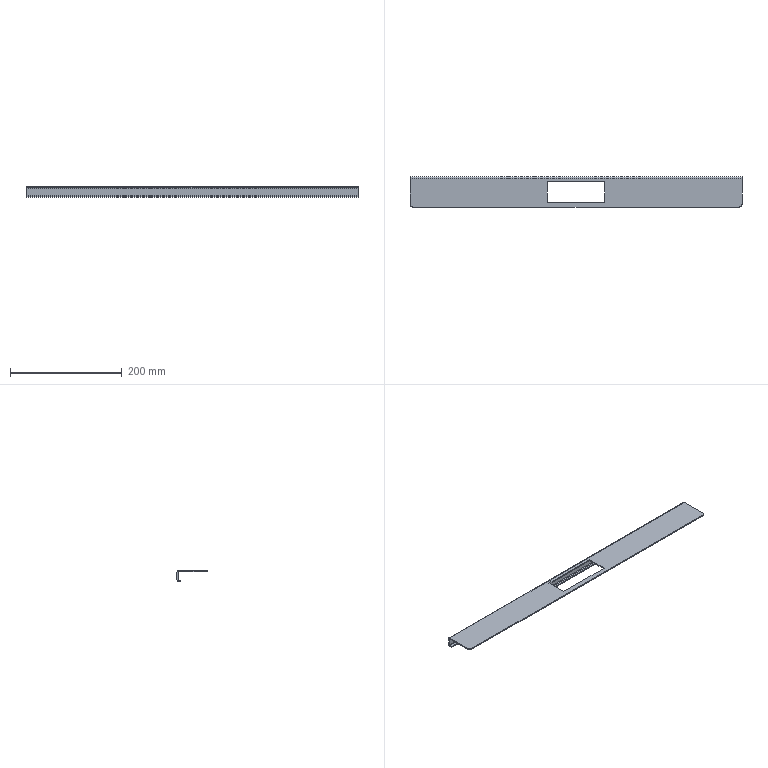Part | NX | 1 solid | 28 faces | box 595 x 54 x 19 mm | volume 80754 mm3 | plane 22 | cylinder 6 | commonest cylinder face diameters 2 x2 6 x2 10 x2
STEP:
#1=CARTESIAN_POINT('',(297.5,48.,87.));
#2=VERTEX_POINT('',#1);
#3=CARTESIAN_POINT('',(297.5,48.,100.));
#4=VERTEX_POINT('',#3);
#5=CARTESIAN_POINT('',(297.5,48.,101.));
#6=DIRECTION('',(0.,0.,1.));
#7=VECTOR('',#6,1000.);
#8=LINE('',#5,#7);
#9=EDGE_CURVE('',#2,#4,#8,.T.);
#10=ORIENTED_EDGE('',*,*,#9,.F.);
#11=CARTESIAN_POINT('',(297.5,50.,87.));
#12=VERTEX_POINT('',#11);
#13=CARTESIAN_POINT('',(297.5,48.,87.));
#14=DIRECTION('',(0.,1.,0.));
#15=VECTOR('',#14,1000.);
#16=LINE('',#13,#15);
#17=EDGE_CURVE('',#2,#12,#16,.T.);
#18=ORIENTED_EDGE('',*,*,#17,.T.);
#19=CARTESIAN_POINT('',(297.5,50.,100.));
#20=VERTEX_POINT('',#19);
#21=CARTESIAN_POINT('',(297.5,50.,101.));
#22=DIRECTION('',(0.,0.,1.));
#23=VECTOR('',#22,1000.);
#24=LINE('',#21,#23);
#25=EDGE_CURVE('',#12,#20,#24,.T.);
#26=ORIENTED_EDGE('',*,*,#25,.T.);
#27=CARTESIAN_POINT('',(297.5,48.,100.));
#28=DIRECTION('',(0.,1.,0.));
#29=VECTOR('',#28,1000.);
#30=LINE('',#27,#29);
#31=EDGE_CURVE('',#4,#20,#30,.T.);
#32=ORIENTED_EDGE('',*,*,#31,.F.);
#33=EDGE_LOOP('',(#10,#18,#26,#32));
#34=FACE_BOUND('',#33,.T.);
#35=CARTESIAN_POINT('',(297.5,50.,101.));
#36=DIRECTION('',(1.,0.,0.));
#37=DIRECTION('',(0.,0.,-1.));
#38=AXIS2_PLACEMENT_3D('',#35,#36,#37);
#39=PLANE('',#38);
#40=ADVANCED_FACE('',(#34),#39,.T.);
#41=ORIENTED_EDGE('',*,*,#25,.F.);
#42=CARTESIAN_POINT('',(-297.5,50.,87.));
#43=VERTEX_POINT('',#42);
#44=CARTESIAN_POINT('',(297.5,50.,87.));
#45=DIRECTION('',(1.,0.,0.));
#46=VECTOR('',#45,1000.);
#47=LINE('',#44,#46);
#48=EDGE_CURVE('',#12,#43,#47,.F.);
#49=ORIENTED_EDGE('',*,*,#48,.T.);
#50=CARTESIAN_POINT('',(-297.5,50.,100.));
#51=VERTEX_POINT('',#50);
#52=CARTESIAN_POINT('',(-297.5,50.,86.));
#53=DIRECTION('',(0.,0.,-1.));
#54=VECTOR('',#53,1000.);
#55=LINE('',#52,#54);
#56=EDGE_CURVE('',#51,#43,#55,.T.);
#57=ORIENTED_EDGE('',*,*,#56,.F.);
#58=CARTESIAN_POINT('',(0.,50.,100.));
#59=DIRECTION('',(1.,0.,0.));
#60=VECTOR('',#59,1000.);
#61=LINE('',#58,#60);
#62=EDGE_CURVE('',#51,#20,#61,.T.);
#63=ORIENTED_EDGE('',*,*,#62,.T.);
#64=EDGE_LOOP('',(#41,#49,#57,#63));
#65=FACE_BOUND('',#64,.T.);
#66=CARTESIAN_POINT('',(0.,50.,0.));
#67=DIRECTION('',(0.,1.,0.));
#68=DIRECTION('',(0.,0.,1.));
#69=AXIS2_PLACEMENT_3D('',#66,#67,#68);
#70=PLANE('',#69);
#71=ADVANCED_FACE('',(#65),#70,.T.);
#72=CARTESIAN_POINT('',(-297.5,48.,87.));
#73=VERTEX_POINT('',#72);
#74=CARTESIAN_POINT('',(297.5,48.,87.));
#75=DIRECTION('',(1.,0.,0.));
#76=VECTOR('',#75,1000.);
#77=LINE('',#74,#76);
#78=EDGE_CURVE('',#2,#73,#77,.F.);
#79=ORIENTED_EDGE('',*,*,#78,.F.);
#80=ORIENTED_EDGE('',*,*,#9,.T.);
#81=CARTESIAN_POINT('',(-297.5,48.,100.));
#82=VERTEX_POINT('',#81);
#83=CARTESIAN_POINT('',(-297.5,48.,100.));
#84=DIRECTION('',(1.,0.,0.));
#85=VECTOR('',#84,1000.);
#86=LINE('',#83,#85);
#87=EDGE_CURVE('',#82,#4,#86,.T.);
#88=ORIENTED_EDGE('',*,*,#87,.F.);
#89=CARTESIAN_POINT('',(-297.5,48.,86.));
#90=DIRECTION('',(0.,0.,-1.));
#91=VECTOR('',#90,1000.);
#92=LINE('',#89,#91);
#93=EDGE_CURVE('',#82,#73,#92,.T.);
#94=ORIENTED_EDGE('',*,*,#93,.T.);
#95=EDGE_LOOP('',(#79,#80,#88,#94));
#96=FACE_BOUND('',#95,.T.);
#97=CARTESIAN_POINT('',(0.,48.,0.));
#98=DIRECTION('',(0.,1.,0.));
#99=DIRECTION('',(0.,0.,1.));
#100=AXIS2_PLACEMENT_3D('',#97,#98,#99);
#101=PLANE('',#100);
#102=ADVANCED_FACE('',(#96),#101,.F.);
#103=CARTESIAN_POINT('',(297.5,1.,103.));
#104=VERTEX_POINT('',#103);
#105=CARTESIAN_POINT('',(297.5,47.,103.));
#106=VERTEX_POINT('',#105);
#107=CARTESIAN_POINT('',(297.5,48.,103.));
#108=DIRECTION('',(0.,1.,0.));
#109=VECTOR('',#108,1000.);
#110=LINE('',#107,#109);
#111=EDGE_CURVE('',#104,#106,#110,.T.);
#112=ORIENTED_EDGE('',*,*,#111,.F.);
#113=CARTESIAN_POINT('',(297.5,1.,101.));
#114=VERTEX_POINT('',#113);
#115=CARTESIAN_POINT('',(297.5,1.,103.));
#116=DIRECTION('',(0.,0.,-1.));
#117=VECTOR('',#116,1000.);
#118=LINE('',#115,#117);
#119=EDGE_CURVE('',#104,#114,#118,.T.);
#120=ORIENTED_EDGE('',*,*,#119,.T.);
#121=CARTESIAN_POINT('',(297.5,47.,101.));
#122=VERTEX_POINT('',#121);
#123=CARTESIAN_POINT('',(297.5,48.,101.));
#124=DIRECTION('',(0.,1.,0.));
#125=VECTOR('',#124,1000.);
#126=LINE('',#123,#125);
#127=EDGE_CURVE('',#114,#122,#126,.T.);
#128=ORIENTED_EDGE('',*,*,#127,.T.);
#129=CARTESIAN_POINT('',(297.5,47.,101.));
#130=DIRECTION('',(0.,0.,1.));
#131=VECTOR('',#130,1000.);
#132=LINE('',#129,#131);
#133=EDGE_CURVE('',#122,#106,#132,.T.);
#134=ORIENTED_EDGE('',*,*,#133,.T.);
#135=EDGE_LOOP('',(#112,#120,#128,#134));
#136=FACE_BOUND('',#135,.T.);
#137=CARTESIAN_POINT('',(297.5,48.,103.));
#138=DIRECTION('',(-1.,0.,0.));
#139=DIRECTION('',(0.,0.,1.));
#140=AXIS2_PLACEMENT_3D('',#137,#138,#139);
#141=PLANE('',#140);
#142=ADVANCED_FACE('',(#136),#141,.F.);
#143=CARTESIAN_POINT('',(-297.5,47.,101.));
#144=VERTEX_POINT('',#143);
#145=CARTESIAN_POINT('',(-297.5,1.,101.));
#146=VERTEX_POINT('',#145);
#147=CARTESIAN_POINT('',(-297.5,48.,101.));
#148=DIRECTION('',(0.,-1.,0.));
#149=VECTOR('',#148,1000.);
#150=LINE('',#147,#149);
#151=EDGE_CURVE('',#144,#146,#150,.T.);
#152=ORIENTED_EDGE('',*,*,#151,.T.);
#153=CARTESIAN_POINT('',(-297.5,1.,103.));
#154=VERTEX_POINT('',#153);
#155=CARTESIAN_POINT('',(-297.5,1.,103.));
#156=DIRECTION('',(0.,0.,-1.));
#157=VECTOR('',#156,1000.);
#158=LINE('',#155,#157);
#159=EDGE_CURVE('',#146,#154,#158,.F.);
#160=ORIENTED_EDGE('',*,*,#159,.T.);
#161=CARTESIAN_POINT('',(-297.5,47.,103.));
#162=VERTEX_POINT('',#161);
#163=CARTESIAN_POINT('',(-297.5,48.,103.));
#164=DIRECTION('',(0.,-1.,0.));
#165=VECTOR('',#164,1000.);
#166=LINE('',#163,#165);
#167=EDGE_CURVE('',#162,#154,#166,.T.);
#168=ORIENTED_EDGE('',*,*,#167,.F.);
#169=CARTESIAN_POINT('',(-297.5,47.,101.));
#170=DIRECTION('',(0.,0.,1.));
#171=VECTOR('',#170,1000.);
#172=LINE('',#169,#171);
#173=EDGE_CURVE('',#144,#162,#172,.T.);
#174=ORIENTED_EDGE('',*,*,#173,.F.);
#175=EDGE_LOOP('',(#152,#160,#168,#174));
#176=FACE_BOUND('',#175,.T.);
#177=CARTESIAN_POINT('',(-297.5,48.,103.));
#178=DIRECTION('',(1.,0.,0.));
#179=DIRECTION('',(0.,0.,-1.));
#180=AXIS2_PLACEMENT_3D('',#177,#178,#179);
#181=PLANE('',#180);
#182=ADVANCED_FACE('',(#176),#181,.F.);
#183=CARTESIAN_POINT('',(-51.5,41.5,103.));
#184=VERTEX_POINT('',#183);
#185=CARTESIAN_POINT('',(-51.5,4.5,103.));
#186=VERTEX_POINT('',#185);
#187=CARTESIAN_POINT('',(-51.5,4.5,103.));
#188=DIRECTION('',(0.,-1.,0.));
#189=VECTOR('',#188,1000.);
#190=LINE('',#187,#189);
#191=EDGE_CURVE('',#184,#186,#190,.T.);
#192=ORIENTED_EDGE('',*,*,#191,.F.);
#193=CARTESIAN_POINT('',(51.5,41.5,103.));
#194=VERTEX_POINT('',#193);
#195=CARTESIAN_POINT('',(51.5,41.5,103.));
#196=DIRECTION('',(-1.,0.,0.));
#197=VECTOR('',#196,1000.);
#198=LINE('',#195,#197);
#199=EDGE_CURVE('',#194,#184,#198,.T.);
#200=ORIENTED_EDGE('',*,*,#199,.F.);
#201=CARTESIAN_POINT('',(51.5,4.5,103.));
#202=VERTEX_POINT('',#201);
#203=CARTESIAN_POINT('',(51.5,4.5,103.));
#204=DIRECTION('',(0.,1.,0.));
#205=VECTOR('',#204,1000.);
#206=LINE('',#203,#205);
#207=EDGE_CURVE('',#202,#194,#206,.T.);
#208=ORIENTED_EDGE('',*,*,#207,.F.);
#209=CARTESIAN_POINT('',(51.5,4.5,103.));
#210=DIRECTION('',(1.,0.,0.));
#211=VECTOR('',#210,1000.);
#212=LINE('',#209,#211);
#213=EDGE_CURVE('',#186,#202,#212,.T.);
#214=ORIENTED_EDGE('',*,*,#213,.F.);
#215=EDGE_LOOP('',(#192,#200,#208,#214));
#216=FACE_BOUND('',#215,.T.);
#217=CARTESIAN_POINT('',(-292.5,-4.,103.));
#218=VERTEX_POINT('',#217);
#219=CARTESIAN_POINT('',(292.5,-4.,103.));
#220=VERTEX_POINT('',#219);
#221=CARTESIAN_POINT('',(-297.5,-4.,103.));
#222=DIRECTION('',(1.,0.,0.));
#223=VECTOR('',#222,1000.);
#224=LINE('',#221,#223);
#225=EDGE_CURVE('',#218,#220,#224,.T.);
#226=ORIENTED_EDGE('',*,*,#225,.T.);
#227=CARTESIAN_POINT('',(292.5,1.,103.));
#228=DIRECTION('',(0.,0.,1.));
#229=DIRECTION('',(1.,0.,0.));
#230=AXIS2_PLACEMENT_3D('',#227,#228,#229);
#231=CIRCLE('',#230,5.);
#232=EDGE_CURVE('',#220,#104,#231,.T.);
#233=ORIENTED_EDGE('',*,*,#232,.T.);
#234=ORIENTED_EDGE('',*,*,#111,.T.);
#235=CARTESIAN_POINT('',(297.5,47.,103.));
#236=DIRECTION('',(1.,0.,0.));
#237=VECTOR('',#236,1000.);
#238=LINE('',#235,#237);
#239=EDGE_CURVE('',#106,#162,#238,.F.);
#240=ORIENTED_EDGE('',*,*,#239,.T.);
#241=ORIENTED_EDGE('',*,*,#167,.T.);
#242=CARTESIAN_POINT('',(-292.5,1.,103.));
#243=DIRECTION('',(0.,0.,1.));
#244=DIRECTION('',(1.,0.,0.));
#245=AXIS2_PLACEMENT_3D('',#242,#243,#244);
#246=CIRCLE('',#245,5.);
#247=EDGE_CURVE('',#154,#218,#246,.T.);
#248=ORIENTED_EDGE('',*,*,#247,.T.);
#249=EDGE_LOOP('',(#226,#233,#234,#240,#241,#248));
#250=FACE_BOUND('',#249,.T.);
#251=CARTESIAN_POINT('',(0.,0.,103.));
#252=DIRECTION('',(0.,0.,1.));
#253=DIRECTION('',(1.,0.,0.));
#254=AXIS2_PLACEMENT_3D('',#251,#252,#253);
#255=PLANE('',#254);
#256=ADVANCED_FACE('',(#216,#250),#255,.T.);
#257=CARTESIAN_POINT('',(51.5,41.5,101.));
#258=VERTEX_POINT('',#257);
#259=CARTESIAN_POINT('',(-51.5,41.5,101.));
#260=VERTEX_POINT('',#259);
#261=CARTESIAN_POINT('',(0.,41.5,101.));
#262=DIRECTION('',(-1.,0.,0.));
#263=VECTOR('',#262,1000.);
#264=LINE('',#261,#263);
#265=EDGE_CURVE('',#258,#260,#264,.T.);
#266=ORIENTED_EDGE('',*,*,#265,.T.);
#267=CARTESIAN_POINT('',(-51.5,4.5,101.));
#268=VERTEX_POINT('',#267);
#269=CARTESIAN_POINT('',(-51.5,0.,101.));
#270=DIRECTION('',(0.,-1.,0.));
#271=VECTOR('',#270,1000.);
#272=LINE('',#269,#271);
#273=EDGE_CURVE('',#260,#268,#272,.T.);
#274=ORIENTED_EDGE('',*,*,#273,.T.);
#275=CARTESIAN_POINT('',(51.5,4.5,101.));
#276=VERTEX_POINT('',#275);
#277=CARTESIAN_POINT('',(0.,4.5,101.));
#278=DIRECTION('',(1.,0.,0.));
#279=VECTOR('',#278,1000.);
#280=LINE('',#277,#279);
#281=EDGE_CURVE('',#268,#276,#280,.T.);
#282=ORIENTED_EDGE('',*,*,#281,.T.);
#283=CARTESIAN_POINT('',(51.5,0.,101.));
#284=DIRECTION('',(0.,1.,0.));
#285=VECTOR('',#284,1000.);
#286=LINE('',#283,#285);
#287=EDGE_CURVE('',#276,#258,#286,.T.);
#288=ORIENTED_EDGE('',*,*,#287,.T.);
#289=EDGE_LOOP('',(#266,#274,#282,#288));
#290=FACE_BOUND('',#289,.T.);
#291=ORIENTED_EDGE('',*,*,#127,.F.);
#292=CARTESIAN_POINT('',(292.5,-4.,101.));
#293=VERTEX_POINT('',#292);
#294=CARTESIAN_POINT('',(292.5,1.,101.));
#295=DIRECTION('',(0.,0.,1.));
#296=DIRECTION('',(1.,0.,0.));
#297=AXIS2_PLACEMENT_3D('',#294,#295,#296);
#298=CIRCLE('',#297,5.);
#299=EDGE_CURVE('',#114,#293,#298,.F.);
#300=ORIENTED_EDGE('',*,*,#299,.T.);
#301=CARTESIAN_POINT('',(-292.5,-4.,101.));
#302=VERTEX_POINT('',#301);
#303=CARTESIAN_POINT('',(-297.5,-4.,101.));
#304=DIRECTION('',(1.,0.,0.));
#305=VECTOR('',#304,1000.);
#306=LINE('',#303,#305);
#307=EDGE_CURVE('',#302,#293,#306,.T.);
#308=ORIENTED_EDGE('',*,*,#307,.F.);
#309=CARTESIAN_POINT('',(-292.5,1.,101.));
#310=DIRECTION('',(0.,0.,1.));
#311=DIRECTION('',(1.,0.,0.));
#312=AXIS2_PLACEMENT_3D('',#309,#310,#311);
#313=CIRCLE('',#312,5.);
#314=EDGE_CURVE('',#302,#146,#313,.F.);
#315=ORIENTED_EDGE('',*,*,#314,.T.);
#316=ORIENTED_EDGE('',*,*,#151,.F.);
#317=CARTESIAN_POINT('',(297.5,47.,101.));
#318=DIRECTION('',(1.,0.,0.));
#319=VECTOR('',#318,1000.);
#320=LINE('',#317,#319);
#321=EDGE_CURVE('',#122,#144,#320,.F.);
#322=ORIENTED_EDGE('',*,*,#321,.F.);
#323=EDGE_LOOP('',(#291,#300,#308,#315,#316,#322));
#324=FACE_BOUND('',#323,.T.);
#325=CARTESIAN_POINT('',(0.,0.,101.));
#326=DIRECTION('',(0.,0.,1.));
#327=DIRECTION('',(1.,0.,0.));
#328=AXIS2_PLACEMENT_3D('',#325,#326,#327);
#329=PLANE('',#328);
#330=ADVANCED_FACE('',(#290,#324),#329,.F.);
#331=ORIENTED_EDGE('',*,*,#307,.T.);
#332=CARTESIAN_POINT('',(292.5,-4.,103.));
#333=DIRECTION('',(0.,0.,-1.));
#334=VECTOR('',#333,1000.);
#335=LINE('',#332,#334);
#336=EDGE_CURVE('',#293,#220,#335,.F.);
#337=ORIENTED_EDGE('',*,*,#336,.T.);
#338=ORIENTED_EDGE('',*,*,#225,.F.);
#339=CARTESIAN_POINT('',(-292.5,-4.,103.));
#340=DIRECTION('',(0.,0.,-1.));
#341=VECTOR('',#340,1000.);
#342=LINE('',#339,#341);
#343=EDGE_CURVE('',#218,#302,#342,.T.);
#344=ORIENTED_EDGE('',*,*,#343,.T.);
#345=EDGE_LOOP('',(#331,#337,#338,#344));
#346=FACE_BOUND('',#345,.T.);
#347=CARTESIAN_POINT('',(-297.5,-4.,103.));
#348=DIRECTION('',(0.,1.,0.));
#349=DIRECTION('',(0.,0.,1.));
#350=AXIS2_PLACEMENT_3D('',#347,#348,#349);
#351=PLANE('',#350);
#352=ADVANCED_FACE('',(#346),#351,.F.);
#353=CARTESIAN_POINT('',(-297.5,48.,100.));
#354=DIRECTION('',(0.,1.,0.));
#355=VECTOR('',#354,1000.);
#356=LINE('',#353,#355);
#357=EDGE_CURVE('',#82,#51,#356,.T.);
#358=ORIENTED_EDGE('',*,*,#357,.F.);
#359=CARTESIAN_POINT('',(-297.5,47.,100.));
#360=DIRECTION('',(1.,0.,0.));
#361=DIRECTION('',(0.,0.,-1.));
#362=AXIS2_PLACEMENT_3D('',#359,#360,#361);
#363=CIRCLE('',#362,1.);
#364=EDGE_CURVE('',#144,#82,#363,.F.);
#365=ORIENTED_EDGE('',*,*,#364,.F.);
#366=ORIENTED_EDGE('',*,*,#173,.T.);
#367=CARTESIAN_POINT('',(-297.5,47.,100.));
#368=DIRECTION('',(1.,0.,0.));
#369=DIRECTION('',(0.,0.,-1.));
#370=AXIS2_PLACEMENT_3D('',#367,#368,#369);
#371=CIRCLE('',#370,3.);
#372=EDGE_CURVE('',#162,#51,#371,.F.);
#373=ORIENTED_EDGE('',*,*,#372,.T.);
#374=EDGE_LOOP('',(#358,#365,#366,#373));
#375=FACE_BOUND('',#374,.T.);
#376=CARTESIAN_POINT('',(-297.5,47.,100.));
#377=DIRECTION('',(-1.,0.,0.));
#378=DIRECTION('',(0.,0.,1.));
#379=AXIS2_PLACEMENT_3D('',#376,#377,#378);
#380=PLANE('',#379);
#381=ADVANCED_FACE('',(#375),#380,.T.);
#382=CARTESIAN_POINT('',(297.5,47.,100.));
#383=DIRECTION('',(1.,0.,0.));
#384=DIRECTION('',(0.,0.,-1.));
#385=AXIS2_PLACEMENT_3D('',#382,#383,#384);
#386=CIRCLE('',#385,1.);
#387=EDGE_CURVE('',#4,#122,#386,.T.);
#388=ORIENTED_EDGE('',*,*,#387,.F.);
#389=ORIENTED_EDGE('',*,*,#31,.T.);
#390=CARTESIAN_POINT('',(297.5,47.,100.));
#391=DIRECTION('',(1.,0.,0.));
#392=DIRECTION('',(0.,0.,-1.));
#393=AXIS2_PLACEMENT_3D('',#390,#391,#392);
#394=CIRCLE('',#393,3.);
#395=EDGE_CURVE('',#20,#106,#394,.T.);
#396=ORIENTED_EDGE('',*,*,#395,.T.);
#397=ORIENTED_EDGE('',*,*,#133,.F.);
#398=EDGE_LOOP('',(#388,#389,#396,#397));
#399=FACE_BOUND('',#398,.T.);
#400=CARTESIAN_POINT('',(297.5,47.,100.));
#401=DIRECTION('',(-1.,0.,0.));
#402=DIRECTION('',(0.,0.,1.));
#403=AXIS2_PLACEMENT_3D('',#400,#401,#402);
#404=PLANE('',#403);
#405=ADVANCED_FACE('',(#399),#404,.F.);
#406=ORIENTED_EDGE('',*,*,#239,.F.);
#407=ORIENTED_EDGE('',*,*,#395,.F.);
#408=ORIENTED_EDGE('',*,*,#62,.F.);
#409=ORIENTED_EDGE('',*,*,#372,.F.);
#410=EDGE_LOOP('',(#406,#407,#408,#409));
#411=FACE_BOUND('',#410,.T.);
#412=CARTESIAN_POINT('',(297.5,47.,100.));
#413=DIRECTION('',(1.,0.,0.));
#414=DIRECTION('',(0.,1.,0.));
#415=AXIS2_PLACEMENT_3D('',#412,#413,#414);
#416=CYLINDRICAL_SURFACE('',#415,3.);
#417=ADVANCED_FACE('',(#411),#416,.T.);
#418=ORIENTED_EDGE('',*,*,#321,.T.);
#419=ORIENTED_EDGE('',*,*,#364,.T.);
#420=ORIENTED_EDGE('',*,*,#87,.T.);
#421=ORIENTED_EDGE('',*,*,#387,.T.);
#422=EDGE_LOOP('',(#418,#419,#420,#421));
#423=FACE_BOUND('',#422,.T.);
#424=CARTESIAN_POINT('',(297.5,47.,100.));
#425=DIRECTION('',(1.,0.,0.));
#426=DIRECTION('',(0.,1.,0.));
#427=AXIS2_PLACEMENT_3D('',#424,#425,#426);
#428=CYLINDRICAL_SURFACE('',#427,1.);
#429=ADVANCED_FACE('',(#423),#428,.F.);
#430=CARTESIAN_POINT('',(-297.5,48.,87.));
#431=DIRECTION('',(0.,1.,0.));
#432=VECTOR('',#431,1000.);
#433=LINE('',#430,#432);
#434=EDGE_CURVE('',#73,#43,#433,.T.);
#435=ORIENTED_EDGE('',*,*,#434,.F.);
#436=ORIENTED_EDGE('',*,*,#93,.F.);
#437=ORIENTED_EDGE('',*,*,#357,.T.);
#438=ORIENTED_EDGE('',*,*,#56,.T.);
#439=EDGE_LOOP('',(#435,#436,#437,#438));
#440=FACE_BOUND('',#439,.T.);
#441=CARTESIAN_POINT('',(-297.5,50.,86.));
#442=DIRECTION('',(-1.,0.,0.));
#443=DIRECTION('',(0.,0.,1.));
#444=AXIS2_PLACEMENT_3D('',#441,#442,#443);
#445=PLANE('',#444);
#446=ADVANCED_FACE('',(#440),#445,.T.);
#447=ORIENTED_EDGE('',*,*,#232,.F.);
#448=ORIENTED_EDGE('',*,*,#336,.F.);
#449=ORIENTED_EDGE('',*,*,#299,.F.);
#450=ORIENTED_EDGE('',*,*,#119,.F.);
#451=EDGE_LOOP('',(#447,#448,#449,#450));
#452=FACE_BOUND('',#451,.T.);
#453=CARTESIAN_POINT('',(292.5,1.,103.));
#454=DIRECTION('',(0.,0.,-1.));
#455=DIRECTION('',(-1.,0.,0.));
#456=AXIS2_PLACEMENT_3D('',#453,#454,#455);
#457=CYLINDRICAL_SURFACE('',#456,5.);
#458=ADVANCED_FACE('',(#452),#457,.T.);
#459=ORIENTED_EDGE('',*,*,#247,.F.);
#460=ORIENTED_EDGE('',*,*,#159,.F.);
#461=ORIENTED_EDGE('',*,*,#314,.F.);
#462=ORIENTED_EDGE('',*,*,#343,.F.);
#463=EDGE_LOOP('',(#459,#460,#461,#462));
#464=FACE_BOUND('',#463,.T.);
#465=CARTESIAN_POINT('',(-292.5,1.,103.));
#466=DIRECTION('',(0.,0.,-1.));
#467=DIRECTION('',(-1.,0.,0.));
#468=AXIS2_PLACEMENT_3D('',#465,#466,#467);
#469=CYLINDRICAL_SURFACE('',#468,5.);
#470=ADVANCED_FACE('',(#464),#469,.T.);
#471=CARTESIAN_POINT('',(-297.5,47.,86.));
#472=VERTEX_POINT('',#471);
#473=CARTESIAN_POINT('',(-297.5,47.,84.));
#474=VERTEX_POINT('',#473);
#475=CARTESIAN_POINT('',(-297.5,47.,86.));
#476=DIRECTION('',(0.,0.,-1.));
#477=VECTOR('',#476,1000.);
#478=LINE('',#475,#477);
#479=EDGE_CURVE('',#472,#474,#478,.T.);
#480=ORIENTED_EDGE('',*,*,#479,.F.);
#481=CARTESIAN_POINT('',(-297.5,47.,87.));
#482=DIRECTION('',(1.,0.,0.));
#483=DIRECTION('',(0.,0.,-1.));
#484=AXIS2_PLACEMENT_3D('',#481,#482,#483);
#485=CIRCLE('',#484,1.);
#486=EDGE_CURVE('',#73,#472,#485,.F.);
#487=ORIENTED_EDGE('',*,*,#486,.F.);
#488=ORIENTED_EDGE('',*,*,#434,.T.);
#489=CARTESIAN_POINT('',(-297.5,47.,87.));
#490=DIRECTION('',(1.,0.,0.));
#491=DIRECTION('',(0.,0.,-1.));
#492=AXIS2_PLACEMENT_3D('',#489,#490,#491);
#493=CIRCLE('',#492,3.);
#494=EDGE_CURVE('',#43,#474,#493,.F.);
#495=ORIENTED_EDGE('',*,*,#494,.T.);
#496=EDGE_LOOP('',(#480,#487,#488,#495));
#497=FACE_BOUND('',#496,.T.);
#498=CARTESIAN_POINT('',(-297.5,47.,87.));
#499=DIRECTION('',(-1.,0.,0.));
#500=DIRECTION('',(0.,0.,1.));
#501=AXIS2_PLACEMENT_3D('',#498,#499,#500);
#502=PLANE('',#501);
#503=ADVANCED_FACE('',(#497),#502,.T.);
#504=CARTESIAN_POINT('',(297.5,47.,86.));
#505=VERTEX_POINT('',#504);
#506=CARTESIAN_POINT('',(297.5,47.,87.));
#507=DIRECTION('',(1.,0.,0.));
#508=DIRECTION('',(0.,0.,-1.));
#509=AXIS2_PLACEMENT_3D('',#506,#507,#508);
#510=CIRCLE('',#509,1.);
#511=EDGE_CURVE('',#505,#2,#510,.T.);
#512=ORIENTED_EDGE('',*,*,#511,.F.);
#513=CARTESIAN_POINT('',(297.5,47.,84.));
#514=VERTEX_POINT('',#513);
#515=CARTESIAN_POINT('',(297.5,47.,86.));
#516=DIRECTION('',(0.,0.,-1.));
#517=VECTOR('',#516,1000.);
#518=LINE('',#515,#517);
#519=EDGE_CURVE('',#505,#514,#518,.T.);
#520=ORIENTED_EDGE('',*,*,#519,.T.);
#521=CARTESIAN_POINT('',(297.5,47.,87.));
#522=DIRECTION('',(1.,0.,0.));
#523=DIRECTION('',(0.,0.,-1.));
#524=AXIS2_PLACEMENT_3D('',#521,#522,#523);
#525=CIRCLE('',#524,3.);
#526=EDGE_CURVE('',#514,#12,#525,.T.);
#527=ORIENTED_EDGE('',*,*,#526,.T.);
#528=ORIENTED_EDGE('',*,*,#17,.F.);
#529=EDGE_LOOP('',(#512,#520,#527,#528));
#530=FACE_BOUND('',#529,.T.);
#531=CARTESIAN_POINT('',(297.5,47.,87.));
#532=DIRECTION('',(-1.,0.,0.));
#533=DIRECTION('',(0.,0.,1.));
#534=AXIS2_PLACEMENT_3D('',#531,#532,#533);
#535=PLANE('',#534);
#536=ADVANCED_FACE('',(#530),#535,.F.);
#537=ORIENTED_EDGE('',*,*,#48,.F.);
#538=ORIENTED_EDGE('',*,*,#526,.F.);
#539=CARTESIAN_POINT('',(0.,47.,84.));
#540=DIRECTION('',(1.,0.,0.));
#541=VECTOR('',#540,1000.);
#542=LINE('',#539,#541);
#543=EDGE_CURVE('',#474,#514,#542,.T.);
#544=ORIENTED_EDGE('',*,*,#543,.F.);
#545=ORIENTED_EDGE('',*,*,#494,.F.);
#546=EDGE_LOOP('',(#537,#538,#544,#545));
#547=FACE_BOUND('',#546,.T.);
#548=CARTESIAN_POINT('',(297.5,47.,87.));
#549=DIRECTION('',(1.,0.,0.));
#550=DIRECTION('',(0.,0.,-1.));
#551=AXIS2_PLACEMENT_3D('',#548,#549,#550);
#552=CYLINDRICAL_SURFACE('',#551,3.);
#553=ADVANCED_FACE('',(#547),#552,.T.);
#554=ORIENTED_EDGE('',*,*,#78,.T.);
#555=ORIENTED_EDGE('',*,*,#486,.T.);
#556=CARTESIAN_POINT('',(-297.5,47.,86.));
#557=DIRECTION('',(1.,0.,0.));
#558=VECTOR('',#557,1000.);
#559=LINE('',#556,#558);
#560=EDGE_CURVE('',#472,#505,#559,.T.);
#561=ORIENTED_EDGE('',*,*,#560,.T.);
#562=ORIENTED_EDGE('',*,*,#511,.T.);
#563=EDGE_LOOP('',(#554,#555,#561,#562));
#564=FACE_BOUND('',#563,.T.);
#565=CARTESIAN_POINT('',(297.5,47.,87.));
#566=DIRECTION('',(1.,0.,0.));
#567=DIRECTION('',(0.,0.,-1.));
#568=AXIS2_PLACEMENT_3D('',#565,#566,#567);
#569=CYLINDRICAL_SURFACE('',#568,1.);
#570=ADVANCED_FACE('',(#564),#569,.F.);
#571=CARTESIAN_POINT('',(297.5,43.,84.));
#572=VERTEX_POINT('',#571);
#573=CARTESIAN_POINT('',(297.5,48.,84.));
#574=DIRECTION('',(0.,1.,0.));
#575=VECTOR('',#574,1000.);
#576=LINE('',#573,#575);
#577=EDGE_CURVE('',#572,#514,#576,.T.);
#578=ORIENTED_EDGE('',*,*,#577,.T.);
#579=ORIENTED_EDGE('',*,*,#519,.F.);
#580=CARTESIAN_POINT('',(297.5,43.,86.));
#581=VERTEX_POINT('',#580);
#582=CARTESIAN_POINT('',(297.5,48.,86.));
#583=DIRECTION('',(0.,1.,0.));
#584=VECTOR('',#583,1000.);
#585=LINE('',#582,#584);
#586=EDGE_CURVE('',#581,#505,#585,.T.);
#587=ORIENTED_EDGE('',*,*,#586,.F.);
#588=CARTESIAN_POINT('',(297.5,43.,84.));
#589=DIRECTION('',(0.,0.,1.));
#590=VECTOR('',#589,1000.);
#591=LINE('',#588,#590);
#592=EDGE_CURVE('',#572,#581,#591,.T.);
#593=ORIENTED_EDGE('',*,*,#592,.F.);
#594=EDGE_LOOP('',(#578,#579,#587,#593));
#595=FACE_BOUND('',#594,.T.);
#596=CARTESIAN_POINT('',(297.5,48.,84.));
#597=DIRECTION('',(1.,0.,0.));
#598=DIRECTION('',(0.,0.,-1.));
#599=AXIS2_PLACEMENT_3D('',#596,#597,#598);
#600=PLANE('',#599);
#601=ADVANCED_FACE('',(#595),#600,.T.);
#602=CARTESIAN_POINT('',(-297.5,43.,86.));
#603=VERTEX_POINT('',#602);
#604=CARTESIAN_POINT('',(-297.5,43.,86.));
#605=DIRECTION('',(0.,-1.,0.));
#606=VECTOR('',#605,1000.);
#607=LINE('',#604,#606);
#608=EDGE_CURVE('',#472,#603,#607,.T.);
#609=ORIENTED_EDGE('',*,*,#608,.F.);
#610=ORIENTED_EDGE('',*,*,#479,.T.);
#611=CARTESIAN_POINT('',(-297.5,43.,84.));
#612=VERTEX_POINT('',#611);
#613=CARTESIAN_POINT('',(-297.5,43.,84.));
#614=DIRECTION('',(0.,-1.,0.));
#615=VECTOR('',#614,1000.);
#616=LINE('',#613,#615);
#617=EDGE_CURVE('',#474,#612,#616,.T.);
#618=ORIENTED_EDGE('',*,*,#617,.T.);
#619=CARTESIAN_POINT('',(-297.5,43.,84.));
#620=DIRECTION('',(0.,0.,1.));
#621=VECTOR('',#620,1000.);
#622=LINE('',#619,#621);
#623=EDGE_CURVE('',#612,#603,#622,.T.);
#624=ORIENTED_EDGE('',*,*,#623,.T.);
#625=EDGE_LOOP('',(#609,#610,#618,#624));
#626=FACE_BOUND('',#625,.T.);
#627=CARTESIAN_POINT('',(-297.5,43.,84.));
#628=DIRECTION('',(-1.,0.,0.));
#629=DIRECTION('',(0.,0.,1.));
#630=AXIS2_PLACEMENT_3D('',#627,#628,#629);
#631=PLANE('',#630);
#632=ADVANCED_FACE('',(#626),#631,.T.);
#633=ORIENTED_EDGE('',*,*,#617,.F.);
#634=ORIENTED_EDGE('',*,*,#543,.T.);
#635=ORIENTED_EDGE('',*,*,#577,.F.);
#636=CARTESIAN_POINT('',(297.5,43.,84.));
#637=DIRECTION('',(1.,0.,0.));
#638=VECTOR('',#637,1000.);
#639=LINE('',#636,#638);
#640=EDGE_CURVE('',#612,#572,#639,.T.);
#641=ORIENTED_EDGE('',*,*,#640,.F.);
#642=EDGE_LOOP('',(#633,#634,#635,#641));
#643=FACE_BOUND('',#642,.T.);
#644=CARTESIAN_POINT('',(0.,0.,84.));
#645=DIRECTION('',(0.,0.,-1.));
#646=DIRECTION('',(0.,1.,0.));
#647=AXIS2_PLACEMENT_3D('',#644,#645,#646);
#648=PLANE('',#647);
#649=ADVANCED_FACE('',(#643),#648,.T.);
#650=ORIENTED_EDGE('',*,*,#560,.F.);
#651=ORIENTED_EDGE('',*,*,#608,.T.);
#652=CARTESIAN_POINT('',(297.5,43.,86.));
#653=DIRECTION('',(1.,0.,0.));
#654=VECTOR('',#653,1000.);
#655=LINE('',#652,#654);
#656=EDGE_CURVE('',#603,#581,#655,.T.);
#657=ORIENTED_EDGE('',*,*,#656,.T.);
#658=ORIENTED_EDGE('',*,*,#586,.T.);
#659=EDGE_LOOP('',(#650,#651,#657,#658));
#660=FACE_BOUND('',#659,.T.);
#661=CARTESIAN_POINT('',(0.,0.,86.));
#662=DIRECTION('',(0.,0.,-1.));
#663=DIRECTION('',(0.,1.,0.));
#664=AXIS2_PLACEMENT_3D('',#661,#662,#663);
#665=PLANE('',#664);
#666=ADVANCED_FACE('',(#660),#665,.F.);
#667=ORIENTED_EDGE('',*,*,#656,.F.);
#668=ORIENTED_EDGE('',*,*,#623,.F.);
#669=ORIENTED_EDGE('',*,*,#640,.T.);
#670=ORIENTED_EDGE('',*,*,#592,.T.);
#671=EDGE_LOOP('',(#667,#668,#669,#670));
#672=FACE_BOUND('',#671,.T.);
#673=CARTESIAN_POINT('',(297.5,43.,84.));
#674=DIRECTION('',(0.,-1.,0.));
#675=DIRECTION('',(0.,0.,-1.));
#676=AXIS2_PLACEMENT_3D('',#673,#674,#675);
#677=PLANE('',#676);
#678=ADVANCED_FACE('',(#672),#677,.T.);
#679=CARTESIAN_POINT('',(-51.5,41.5,63.));
#680=DIRECTION('',(0.,0.,1.));
#681=VECTOR('',#680,1000.);
#682=LINE('',#679,#681);
#683=EDGE_CURVE('',#260,#184,#682,.T.);
#684=ORIENTED_EDGE('',*,*,#683,.T.);
#685=ORIENTED_EDGE('',*,*,#191,.T.);
#686=CARTESIAN_POINT('',(-51.5,4.5,63.));
#687=DIRECTION('',(0.,0.,1.));
#688=VECTOR('',#687,1000.);
#689=LINE('',#686,#688);
#690=EDGE_CURVE('',#268,#186,#689,.T.);
#691=ORIENTED_EDGE('',*,*,#690,.F.);
#692=ORIENTED_EDGE('',*,*,#273,.F.);
#693=EDGE_LOOP('',(#684,#685,#691,#692));
#694=FACE_BOUND('',#693,.T.);
#695=CARTESIAN_POINT('',(-51.5,4.5,63.));
#696=DIRECTION('',(-1.,0.,0.));
#697=DIRECTION('',(0.,0.,1.));
#698=AXIS2_PLACEMENT_3D('',#695,#696,#697);
#699=PLANE('',#698);
#700=ADVANCED_FACE('',(#694),#699,.F.);
#701=CARTESIAN_POINT('',(51.5,41.5,63.));
#702=DIRECTION('',(0.,0.,1.));
#703=VECTOR('',#702,1000.);
#704=LINE('',#701,#703);
#705=EDGE_CURVE('',#258,#194,#704,.T.);
#706=ORIENTED_EDGE('',*,*,#705,.T.);
#707=ORIENTED_EDGE('',*,*,#199,.T.);
#708=ORIENTED_EDGE('',*,*,#683,.F.);
#709=ORIENTED_EDGE('',*,*,#265,.F.);
#710=EDGE_LOOP('',(#706,#707,#708,#709));
#711=FACE_BOUND('',#710,.T.);
#712=CARTESIAN_POINT('',(51.5,41.5,63.));
#713=DIRECTION('',(0.,1.,0.));
#714=DIRECTION('',(-1.,0.,0.));
#715=AXIS2_PLACEMENT_3D('',#712,#713,#714);
#716=PLANE('',#715);
#717=ADVANCED_FACE('',(#711),#716,.F.);
#718=CARTESIAN_POINT('',(51.5,4.5,63.));
#719=DIRECTION('',(0.,0.,1.));
#720=VECTOR('',#719,1000.);
#721=LINE('',#718,#720);
#722=EDGE_CURVE('',#276,#202,#721,.T.);
#723=ORIENTED_EDGE('',*,*,#722,.T.);
#724=ORIENTED_EDGE('',*,*,#207,.T.);
#725=ORIENTED_EDGE('',*,*,#705,.F.);
#726=ORIENTED_EDGE('',*,*,#287,.F.);
#727=EDGE_LOOP('',(#723,#724,#725,#726));
#728=FACE_BOUND('',#727,.T.);
#729=CARTESIAN_POINT('',(51.5,4.5,63.));
#730=DIRECTION('',(1.,0.,0.));
#731=DIRECTION('',(0.,0.,-1.));
#732=AXIS2_PLACEMENT_3D('',#729,#730,#731);
#733=PLANE('',#732);
#734=ADVANCED_FACE('',(#728),#733,.F.);
#735=ORIENTED_EDGE('',*,*,#690,.T.);
#736=ORIENTED_EDGE('',*,*,#213,.T.);
#737=ORIENTED_EDGE('',*,*,#722,.F.);
#738=ORIENTED_EDGE('',*,*,#281,.F.);
#739=EDGE_LOOP('',(#735,#736,#737,#738));
#740=FACE_BOUND('',#739,.T.);
#741=CARTESIAN_POINT('',(51.5,4.5,63.));
#742=DIRECTION('',(0.,-1.,0.));
#743=DIRECTION('',(1.,0.,0.));
#744=AXIS2_PLACEMENT_3D('',#741,#742,#743);
#745=PLANE('',#744);
#746=ADVANCED_FACE('',(#740),#745,.F.);
#747=CLOSED_SHELL('',(#40,#71,#102,#142,#182,#256,#330,#352,#381,#405,#417,#429,#446,#458,#470,#503,#536,#553,#570,#601,#632,#649,#666,#678,#700,#717,#734,#746));
#748=MANIFOLD_SOLID_BREP('',#747);
#749=(LENGTH_UNIT()NAMED_UNIT(*)SI_UNIT(.MILLI.,.METRE.));
#750=UNCERTAINTY_MEASURE_WITH_UNIT(LENGTH_MEASURE(0.00001),#749,'','');
#751=(NAMED_UNIT(*)PLANE_ANGLE_UNIT()SI_UNIT($,.RADIAN.));
#752=(NAMED_UNIT(*)SI_UNIT($,.STERADIAN.)SOLID_ANGLE_UNIT());
#753=(GEOMETRIC_REPRESENTATION_CONTEXT(3)GLOBAL_UNCERTAINTY_ASSIGNED_CONTEXT((#750))GLOBAL_UNIT_ASSIGNED_CONTEXT((#749,#751,#752))REPRESENTATION_CONTEXT('',''));
#754=ADVANCED_BREP_SHAPE_REPRESENTATION('',(#748),#753);